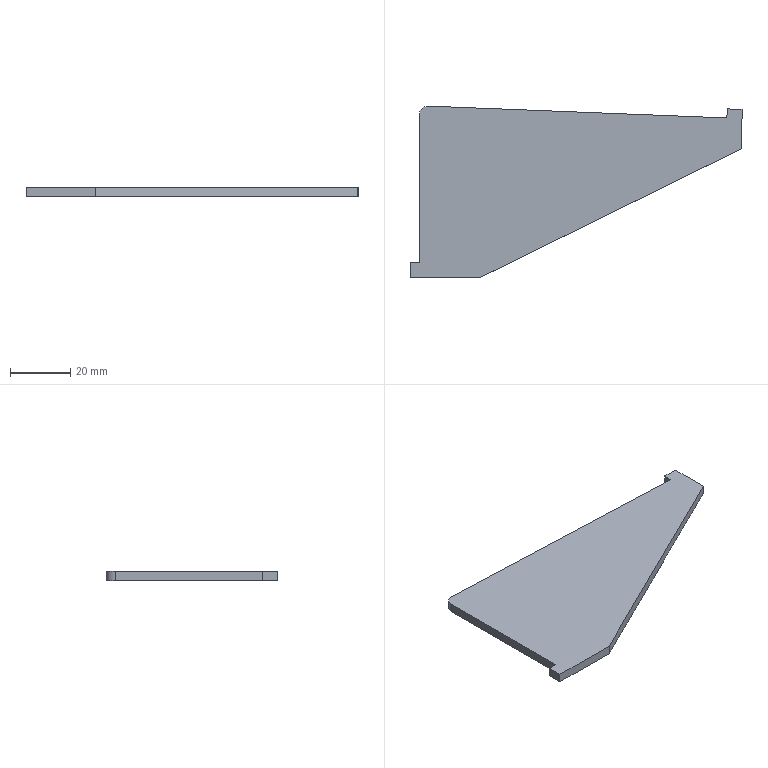Part | STEP file | TS-003-02 | 1 solid | 13 faces | box 109.897 x 56.866 x 3 mm | volume 12102 mm3 | plane 12 | cylinder 1 | commonest cylinder face diameters 6 x1
STEP:
#1=CARTESIAN_POINT('',(0.,0.,0.));
#2=DIRECTION('',(0.,0.,1.));
#3=DIRECTION('',(1.,0.,0.));
#4=AXIS2_PLACEMENT_3D('',#1,#2,#3);
#5=CARTESIAN_POINT('',(-4321.085,3720.403,0.));
#6=VERTEX_POINT('',#5);
#7=CARTESIAN_POINT('',(-4234.241,3763.152,0.));
#8=VERTEX_POINT('',#7);
#9=CARTESIAN_POINT('',(-4234.241,3763.152,0.));
#10=DIRECTION('',(0.8972,0.4416,0.));
#11=VECTOR('',#10,1.);
#12=LINE('',#9,#11);
#13=CARTESIAN_POINT('',(-4234.241,3763.152,-3.));
#14=DIRECTION('',(0.4416,-0.8972,0.));
#15=DIRECTION('',(0.8972,0.4416,0.));
#16=AXIS2_PLACEMENT_3D('',#13,#14,#15);
#17=PLANE('',#16);
#18=CARTESIAN_POINT('',(0.,3.));
#19=DIRECTION('',(1.,0.));
#20=VECTOR('',#19,1.);
#21=LINE('',#18,#20);
#22=(GEOMETRIC_REPRESENTATION_CONTEXT(2)PARAMETRIC_REPRESENTATION_CONTEXT()REPRESENTATION_CONTEXT('',''));
#23=DEFINITIONAL_REPRESENTATION('',(#21),#22);
#24=PCURVE('',#17,#23);
#25=CARTESIAN_POINT('',(-4338.085,3774.268,0.));
#26=DIRECTION('',(0.,0.,-1.));
#27=DIRECTION('',(-1.,0.,0.));
#28=AXIS2_PLACEMENT_3D('',#25,#26,#27);
#29=PLANE('',#28);
#30=CARTESIAN_POINT('',(-103.844,-11.117));
#31=DIRECTION('',(-0.8972,0.4416));
#32=VECTOR('',#31,1.);
#33=LINE('',#30,#32);
#34=(GEOMETRIC_REPRESENTATION_CONTEXT(2)PARAMETRIC_REPRESENTATION_CONTEXT()REPRESENTATION_CONTEXT('',''));
#35=DEFINITIONAL_REPRESENTATION('',(#33),#34);
#36=PCURVE('',#29,#35);
#37=SURFACE_CURVE('',#12,(#24,#36),.PCURVE_S1.);
#38=EDGE_CURVE('',#6,#8,#37,.T.);
#39=ORIENTED_EDGE('',*,*,#38,.F.);
#40=CARTESIAN_POINT('',(-4321.085,3720.403,-3.));
#41=VERTEX_POINT('',#40);
#42=CARTESIAN_POINT('',(-4321.085,3720.403,-3.));
#43=DIRECTION('',(0.,0.,1.));
#44=VECTOR('',#43,1.);
#45=LINE('',#42,#44);
#46=CARTESIAN_POINT('',(-96.795,0.));
#47=DIRECTION('',(0.,1.));
#48=VECTOR('',#47,1.);
#49=LINE('',#46,#48);
#50=(GEOMETRIC_REPRESENTATION_CONTEXT(2)PARAMETRIC_REPRESENTATION_CONTEXT()REPRESENTATION_CONTEXT('',''));
#51=DEFINITIONAL_REPRESENTATION('',(#49),#50);
#52=PCURVE('',#17,#51);
#53=CARTESIAN_POINT('',(-4321.085,3720.403,-3.));
#54=DIRECTION('',(0.,-1.,0.));
#55=DIRECTION('',(0.,0.,-1.));
#56=AXIS2_PLACEMENT_3D('',#53,#54,#55);
#57=PLANE('',#56);
#58=CARTESIAN_POINT('',(0.,0.));
#59=DIRECTION('',(-1.,0.));
#60=VECTOR('',#59,1.);
#61=LINE('',#58,#60);
#62=(GEOMETRIC_REPRESENTATION_CONTEXT(2)PARAMETRIC_REPRESENTATION_CONTEXT()REPRESENTATION_CONTEXT('',''));
#63=DEFINITIONAL_REPRESENTATION('',(#61),#62);
#64=PCURVE('',#57,#63);
#65=SURFACE_CURVE('',#45,(#52,#64),.PCURVE_S1.);
#66=EDGE_CURVE('',#41,#6,#65,.T.);
#67=ORIENTED_EDGE('',*,*,#66,.F.);
#68=CARTESIAN_POINT('',(-4234.241,3763.152,-3.));
#69=VERTEX_POINT('',#68);
#70=CARTESIAN_POINT('',(-4234.241,3763.152,-3.));
#71=DIRECTION('',(0.8972,0.4416,0.));
#72=VECTOR('',#71,1.);
#73=LINE('',#70,#72);
#74=CARTESIAN_POINT('',(0.,0.));
#75=DIRECTION('',(1.,0.));
#76=VECTOR('',#75,1.);
#77=LINE('',#74,#76);
#78=(GEOMETRIC_REPRESENTATION_CONTEXT(2)PARAMETRIC_REPRESENTATION_CONTEXT()REPRESENTATION_CONTEXT('',''));
#79=DEFINITIONAL_REPRESENTATION('',(#77),#78);
#80=PCURVE('',#17,#79);
#81=CARTESIAN_POINT('',(-4338.085,3774.268,-3.));
#82=DIRECTION('',(0.,0.,-1.));
#83=DIRECTION('',(-1.,0.,0.));
#84=AXIS2_PLACEMENT_3D('',#81,#82,#83);
#85=PLANE('',#84);
#86=CARTESIAN_POINT('',(-103.844,-11.117));
#87=DIRECTION('',(-0.8972,0.4416));
#88=VECTOR('',#87,1.);
#89=LINE('',#86,#88);
#90=(GEOMETRIC_REPRESENTATION_CONTEXT(2)PARAMETRIC_REPRESENTATION_CONTEXT()REPRESENTATION_CONTEXT('',''));
#91=DEFINITIONAL_REPRESENTATION('',(#89),#90);
#92=PCURVE('',#85,#91);
#93=SURFACE_CURVE('',#73,(#80,#92),.PCURVE_S1.);
#94=EDGE_CURVE('',#41,#69,#93,.T.);
#95=ORIENTED_EDGE('',*,*,#94,.T.);
#96=CARTESIAN_POINT('',(-4234.241,3763.152,-3.));
#97=DIRECTION('',(0.,0.,1.));
#98=VECTOR('',#97,1.);
#99=LINE('',#96,#98);
#100=CARTESIAN_POINT('',(0.,0.));
#101=DIRECTION('',(0.,1.));
#102=VECTOR('',#101,1.);
#103=LINE('',#100,#102);
#104=(GEOMETRIC_REPRESENTATION_CONTEXT(2)PARAMETRIC_REPRESENTATION_CONTEXT()REPRESENTATION_CONTEXT('',''));
#105=DEFINITIONAL_REPRESENTATION('',(#103),#104);
#106=PCURVE('',#17,#105);
#107=CARTESIAN_POINT('',(-4234.188,3773.152,-3.));
#108=DIRECTION('',(1.,-0.005262,0.));
#109=DIRECTION('',(0.005262,1.,0.));
#110=AXIS2_PLACEMENT_3D('',#107,#108,#109);
#111=PLANE('',#110);
#112=CARTESIAN_POINT('',(-10.,0.));
#113=DIRECTION('',(0.,1.));
#114=VECTOR('',#113,1.);
#115=LINE('',#112,#114);
#116=(GEOMETRIC_REPRESENTATION_CONTEXT(2)PARAMETRIC_REPRESENTATION_CONTEXT()REPRESENTATION_CONTEXT('',''));
#117=DEFINITIONAL_REPRESENTATION('',(#115),#116);
#118=PCURVE('',#111,#117);
#119=SURFACE_CURVE('',#99,(#106,#118),.PCURVE_S1.);
#120=EDGE_CURVE('',#69,#8,#119,.T.);
#121=ORIENTED_EDGE('',*,*,#120,.T.);
#122=EDGE_LOOP('',(#39,#67,#95,#121));
#123=FACE_BOUND('',#122,.T.);
#124=ADVANCED_FACE('',(#123),#17,.T.);
#125=CARTESIAN_POINT('',(-4344.085,3720.403,0.));
#126=VERTEX_POINT('',#125);
#127=CARTESIAN_POINT('',(-4321.085,3720.403,0.));
#128=DIRECTION('',(1.,0.,0.));
#129=VECTOR('',#128,1.);
#130=LINE('',#127,#129);
#131=CARTESIAN_POINT('',(-3.,0.));
#132=DIRECTION('',(0.,1.));
#133=VECTOR('',#132,1.);
#134=LINE('',#131,#133);
#135=(GEOMETRIC_REPRESENTATION_CONTEXT(2)PARAMETRIC_REPRESENTATION_CONTEXT()REPRESENTATION_CONTEXT('',''));
#136=DEFINITIONAL_REPRESENTATION('',(#134),#135);
#137=PCURVE('',#57,#136);
#138=CARTESIAN_POINT('',(-17.,-53.866));
#139=DIRECTION('',(-1.,0.));
#140=VECTOR('',#139,1.);
#141=LINE('',#138,#140);
#142=(GEOMETRIC_REPRESENTATION_CONTEXT(2)PARAMETRIC_REPRESENTATION_CONTEXT()REPRESENTATION_CONTEXT('',''));
#143=DEFINITIONAL_REPRESENTATION('',(#141),#142);
#144=PCURVE('',#29,#143);
#145=SURFACE_CURVE('',#130,(#137,#144),.PCURVE_S1.);
#146=EDGE_CURVE('',#126,#6,#145,.T.);
#147=ORIENTED_EDGE('',*,*,#146,.F.);
#148=CARTESIAN_POINT('',(-4344.085,3720.403,-3.));
#149=VERTEX_POINT('',#148);
#150=CARTESIAN_POINT('',(-4344.085,3720.403,-3.));
#151=DIRECTION('',(0.,0.,1.));
#152=VECTOR('',#151,1.);
#153=LINE('',#150,#152);
#154=CARTESIAN_POINT('',(0.,-23.));
#155=DIRECTION('',(-1.,0.));
#156=VECTOR('',#155,1.);
#157=LINE('',#154,#156);
#158=(GEOMETRIC_REPRESENTATION_CONTEXT(2)PARAMETRIC_REPRESENTATION_CONTEXT()REPRESENTATION_CONTEXT('',''));
#159=DEFINITIONAL_REPRESENTATION('',(#157),#158);
#160=PCURVE('',#57,#159);
#161=CARTESIAN_POINT('',(-4344.085,3720.403,-3.));
#162=DIRECTION('',(-1.,0.,0.));
#163=DIRECTION('',(0.,0.,1.));
#164=AXIS2_PLACEMENT_3D('',#161,#162,#163);
#165=PLANE('',#164);
#166=CARTESIAN_POINT('',(0.,0.));
#167=DIRECTION('',(1.,0.));
#168=VECTOR('',#167,1.);
#169=LINE('',#166,#168);
#170=(GEOMETRIC_REPRESENTATION_CONTEXT(2)PARAMETRIC_REPRESENTATION_CONTEXT()REPRESENTATION_CONTEXT('',''));
#171=DEFINITIONAL_REPRESENTATION('',(#169),#170);
#172=PCURVE('',#165,#171);
#173=SURFACE_CURVE('',#153,(#160,#172),.PCURVE_S1.);
#174=EDGE_CURVE('',#149,#126,#173,.T.);
#175=ORIENTED_EDGE('',*,*,#174,.F.);
#176=CARTESIAN_POINT('',(-4321.085,3720.403,-3.));
#177=DIRECTION('',(1.,0.,0.));
#178=VECTOR('',#177,1.);
#179=LINE('',#176,#178);
#180=CARTESIAN_POINT('',(0.,0.));
#181=DIRECTION('',(0.,1.));
#182=VECTOR('',#181,1.);
#183=LINE('',#180,#182);
#184=(GEOMETRIC_REPRESENTATION_CONTEXT(2)PARAMETRIC_REPRESENTATION_CONTEXT()REPRESENTATION_CONTEXT('',''));
#185=DEFINITIONAL_REPRESENTATION('',(#183),#184);
#186=PCURVE('',#57,#185);
#187=CARTESIAN_POINT('',(-17.,-53.866));
#188=DIRECTION('',(-1.,0.));
#189=VECTOR('',#188,1.);
#190=LINE('',#187,#189);
#191=(GEOMETRIC_REPRESENTATION_CONTEXT(2)PARAMETRIC_REPRESENTATION_CONTEXT()REPRESENTATION_CONTEXT('',''));
#192=DEFINITIONAL_REPRESENTATION('',(#190),#191);
#193=PCURVE('',#85,#192);
#194=SURFACE_CURVE('',#179,(#186,#193),.PCURVE_S1.);
#195=EDGE_CURVE('',#149,#41,#194,.T.);
#196=ORIENTED_EDGE('',*,*,#195,.T.);
#197=ORIENTED_EDGE('',*,*,#66,.T.);
#198=EDGE_LOOP('',(#147,#175,#196,#197));
#199=FACE_BOUND('',#198,.T.);
#200=ADVANCED_FACE('',(#199),#57,.T.);
#201=CARTESIAN_POINT('',(-4341.085,3725.403,-3.));
#202=VERTEX_POINT('',#201);
#203=CARTESIAN_POINT('',(-4341.085,3725.403,0.));
#204=VERTEX_POINT('',#203);
#205=CARTESIAN_POINT('',(-4341.085,3725.403,-3.));
#206=DIRECTION('',(0.,0.,1.));
#207=VECTOR('',#206,1.);
#208=LINE('',#205,#207);
#209=CARTESIAN_POINT('',(-4341.085,3720.403,-3.));
#210=DIRECTION('',(-1.,0.,0.));
#211=DIRECTION('',(0.,0.,1.));
#212=AXIS2_PLACEMENT_3D('',#209,#210,#211);
#213=PLANE('',#212);
#214=CARTESIAN_POINT('',(0.,5.));
#215=DIRECTION('',(1.,0.));
#216=VECTOR('',#215,1.);
#217=LINE('',#214,#216);
#218=(GEOMETRIC_REPRESENTATION_CONTEXT(2)PARAMETRIC_REPRESENTATION_CONTEXT()REPRESENTATION_CONTEXT('',''));
#219=DEFINITIONAL_REPRESENTATION('',(#217),#218);
#220=PCURVE('',#213,#219);
#221=CARTESIAN_POINT('',(-4341.085,3725.403,-3.));
#222=DIRECTION('',(0.,1.,0.));
#223=DIRECTION('',(0.,0.,1.));
#224=AXIS2_PLACEMENT_3D('',#221,#222,#223);
#225=PLANE('',#224);
#226=CARTESIAN_POINT('',(0.,0.));
#227=DIRECTION('',(1.,0.));
#228=VECTOR('',#227,1.);
#229=LINE('',#226,#228);
#230=(GEOMETRIC_REPRESENTATION_CONTEXT(2)PARAMETRIC_REPRESENTATION_CONTEXT()REPRESENTATION_CONTEXT('',''));
#231=DEFINITIONAL_REPRESENTATION('',(#229),#230);
#232=PCURVE('',#225,#231);
#233=SURFACE_CURVE('',#208,(#220,#232),.PCURVE_S1.);
#234=EDGE_CURVE('',#202,#204,#233,.T.);
#235=ORIENTED_EDGE('',*,*,#234,.T.);
#236=CARTESIAN_POINT('',(-4341.085,3774.268,0.));
#237=VERTEX_POINT('',#236);
#238=CARTESIAN_POINT('',(-4341.085,3720.403,0.));
#239=DIRECTION('',(0.,-1.,0.));
#240=VECTOR('',#239,1.);
#241=LINE('',#238,#240);
#242=CARTESIAN_POINT('',(3.,0.));
#243=DIRECTION('',(0.,-1.));
#244=VECTOR('',#243,1.);
#245=LINE('',#242,#244);
#246=(GEOMETRIC_REPRESENTATION_CONTEXT(2)PARAMETRIC_REPRESENTATION_CONTEXT()REPRESENTATION_CONTEXT('',''));
#247=DEFINITIONAL_REPRESENTATION('',(#245),#246);
#248=PCURVE('',#213,#247);
#249=CARTESIAN_POINT('',(3.,-53.866));
#250=DIRECTION('',(0.,-1.));
#251=VECTOR('',#250,1.);
#252=LINE('',#249,#251);
#253=(GEOMETRIC_REPRESENTATION_CONTEXT(2)PARAMETRIC_REPRESENTATION_CONTEXT()REPRESENTATION_CONTEXT('',''));
#254=DEFINITIONAL_REPRESENTATION('',(#252),#253);
#255=PCURVE('',#29,#254);
#256=SURFACE_CURVE('',#241,(#248,#255),.PCURVE_S1.);
#257=EDGE_CURVE('',#237,#204,#256,.T.);
#258=ORIENTED_EDGE('',*,*,#257,.F.);
#259=CARTESIAN_POINT('',(-4341.085,3774.268,-3.));
#260=VERTEX_POINT('',#259);
#261=CARTESIAN_POINT('',(-4341.085,3774.268,-3.));
#262=DIRECTION('',(0.,0.,1.));
#263=VECTOR('',#262,1.);
#264=LINE('',#261,#263);
#265=CARTESIAN_POINT('',(0.,53.866));
#266=DIRECTION('',(1.,0.));
#267=VECTOR('',#266,1.);
#268=LINE('',#265,#267);
#269=(GEOMETRIC_REPRESENTATION_CONTEXT(2)PARAMETRIC_REPRESENTATION_CONTEXT()REPRESENTATION_CONTEXT('',''));
#270=DEFINITIONAL_REPRESENTATION('',(#268),#269);
#271=PCURVE('',#213,#270);
#272=CARTESIAN_POINT('',(-4338.085,3774.268,-3.));
#273=DIRECTION('',(0.,0.,1.));
#274=DIRECTION('',(1.,0.,0.));
#275=AXIS2_PLACEMENT_3D('',#272,#273,#274);
#276=CYLINDRICAL_SURFACE('',#275,3.);
#277=CARTESIAN_POINT('',(3.142,0.));
#278=DIRECTION('',(0.,1.));
#279=VECTOR('',#278,1.);
#280=LINE('',#277,#279);
#281=(GEOMETRIC_REPRESENTATION_CONTEXT(2)PARAMETRIC_REPRESENTATION_CONTEXT()REPRESENTATION_CONTEXT('',''));
#282=DEFINITIONAL_REPRESENTATION('',(#280),#281);
#283=PCURVE('',#276,#282);
#284=SURFACE_CURVE('',#264,(#271,#283),.PCURVE_S1.);
#285=EDGE_CURVE('',#260,#237,#284,.T.);
#286=ORIENTED_EDGE('',*,*,#285,.F.);
#287=CARTESIAN_POINT('',(-4341.085,3720.403,-3.));
#288=DIRECTION('',(0.,-1.,0.));
#289=VECTOR('',#288,1.);
#290=LINE('',#287,#289);
#291=CARTESIAN_POINT('',(0.,0.));
#292=DIRECTION('',(0.,-1.));
#293=VECTOR('',#292,1.);
#294=LINE('',#291,#293);
#295=(GEOMETRIC_REPRESENTATION_CONTEXT(2)PARAMETRIC_REPRESENTATION_CONTEXT()REPRESENTATION_CONTEXT('',''));
#296=DEFINITIONAL_REPRESENTATION('',(#294),#295);
#297=PCURVE('',#213,#296);
#298=CARTESIAN_POINT('',(3.,-53.866));
#299=DIRECTION('',(0.,-1.));
#300=VECTOR('',#299,1.);
#301=LINE('',#298,#300);
#302=(GEOMETRIC_REPRESENTATION_CONTEXT(2)PARAMETRIC_REPRESENTATION_CONTEXT()REPRESENTATION_CONTEXT('',''));
#303=DEFINITIONAL_REPRESENTATION('',(#301),#302);
#304=PCURVE('',#85,#303);
#305=SURFACE_CURVE('',#290,(#297,#304),.PCURVE_S1.);
#306=EDGE_CURVE('',#260,#202,#305,.T.);
#307=ORIENTED_EDGE('',*,*,#306,.T.);
#308=EDGE_LOOP('',(#235,#258,#286,#307));
#309=FACE_BOUND('',#308,.T.);
#310=ADVANCED_FACE('',(#309),#213,.T.);
#311=CARTESIAN_POINT('',(-4338.019,3777.268,0.));
#312=VERTEX_POINT('',#311);
#313=CARTESIAN_POINT('',(-4338.085,3774.268,0.));
#314=DIRECTION('',(0.,0.,1.));
#315=DIRECTION('',(-1.,0.,0.));
#316=AXIS2_PLACEMENT_3D('',#313,#314,#315);
#317=CIRCLE('',#316,3.);
#318=CARTESIAN_POINT('',(-3.142,3.));
#319=DIRECTION('',(1.,0.));
#320=VECTOR('',#319,1.);
#321=LINE('',#318,#320);
#322=(GEOMETRIC_REPRESENTATION_CONTEXT(2)PARAMETRIC_REPRESENTATION_CONTEXT()REPRESENTATION_CONTEXT('',''));
#323=DEFINITIONAL_REPRESENTATION('',(#321),#322);
#324=PCURVE('',#276,#323);
#325=CARTESIAN_POINT('',(3.,0.));
#326=CARTESIAN_POINT('',(3.,-5.196));
#327=CARTESIAN_POINT('',(-1.5,-2.598));
#328=CARTESIAN_POINT('',(-6.,0.));
#329=CARTESIAN_POINT('',(-1.5,2.598));
#330=CARTESIAN_POINT('',(3.,5.196));
#331=CARTESIAN_POINT('',(3.,0.));
#332=(BOUNDED_CURVE()B_SPLINE_CURVE(2,(#325,#326,#327,#328,#329,#330,#331),.UNSPECIFIED.,.T.,.F.)B_SPLINE_CURVE_WITH_KNOTS((1,2,2,2,2,1),(-2.094,0.,2.094,4.189,6.283,8.378),.UNSPECIFIED.)CURVE()GEOMETRIC_REPRESENTATION_ITEM()RATIONAL_B_SPLINE_CURVE((1.,0.5,1.,0.5,1.,0.5,1.))REPRESENTATION_ITEM(''));
#333=(GEOMETRIC_REPRESENTATION_CONTEXT(2)PARAMETRIC_REPRESENTATION_CONTEXT()REPRESENTATION_CONTEXT('',''));
#334=DEFINITIONAL_REPRESENTATION('',(#332),#333);
#335=PCURVE('',#29,#334);
#336=SURFACE_CURVE('',#317,(#324,#335),.PCURVE_S1.);
#337=EDGE_CURVE('',#312,#237,#336,.T.);
#338=ORIENTED_EDGE('',*,*,#337,.F.);
#339=CARTESIAN_POINT('',(-4338.019,3777.268,-3.));
#340=VERTEX_POINT('',#339);
#341=CARTESIAN_POINT('',(-4338.019,3777.268,-3.));
#342=DIRECTION('',(0.,0.,1.));
#343=VECTOR('',#342,1.);
#344=LINE('',#341,#343);
#345=CARTESIAN_POINT('',(1.549,0.));
#346=DIRECTION('',(0.,1.));
#347=VECTOR('',#346,1.);
#348=LINE('',#345,#347);
#349=(GEOMETRIC_REPRESENTATION_CONTEXT(2)PARAMETRIC_REPRESENTATION_CONTEXT()REPRESENTATION_CONTEXT('',''));
#350=DEFINITIONAL_REPRESENTATION('',(#348),#349);
#351=PCURVE('',#276,#350);
#352=CARTESIAN_POINT('',(-4338.019,3777.268,-3.));
#353=DIRECTION('',(0.03961,0.9992,0.));
#354=DIRECTION('',(-0.9992,0.03961,0.));
#355=AXIS2_PLACEMENT_3D('',#352,#353,#354);
#356=PLANE('',#355);
#357=CARTESIAN_POINT('',(0.,0.));
#358=DIRECTION('',(0.,1.));
#359=VECTOR('',#358,1.);
#360=LINE('',#357,#359);
#361=(GEOMETRIC_REPRESENTATION_CONTEXT(2)PARAMETRIC_REPRESENTATION_CONTEXT()REPRESENTATION_CONTEXT('',''));
#362=DEFINITIONAL_REPRESENTATION('',(#360),#361);
#363=PCURVE('',#356,#362);
#364=SURFACE_CURVE('',#344,(#351,#363),.PCURVE_S1.);
#365=EDGE_CURVE('',#340,#312,#364,.T.);
#366=ORIENTED_EDGE('',*,*,#365,.F.);
#367=CARTESIAN_POINT('',(-4338.085,3774.268,-3.));
#368=DIRECTION('',(0.,0.,1.));
#369=DIRECTION('',(-1.,0.,0.));
#370=AXIS2_PLACEMENT_3D('',#367,#368,#369);
#371=CIRCLE('',#370,3.);
#372=CARTESIAN_POINT('',(-3.142,0.));
#373=DIRECTION('',(1.,0.));
#374=VECTOR('',#373,1.);
#375=LINE('',#372,#374);
#376=(GEOMETRIC_REPRESENTATION_CONTEXT(2)PARAMETRIC_REPRESENTATION_CONTEXT()REPRESENTATION_CONTEXT('',''));
#377=DEFINITIONAL_REPRESENTATION('',(#375),#376);
#378=PCURVE('',#276,#377);
#379=CARTESIAN_POINT('',(3.,0.));
#380=CARTESIAN_POINT('',(3.,-5.196));
#381=CARTESIAN_POINT('',(-1.5,-2.598));
#382=CARTESIAN_POINT('',(-6.,0.));
#383=CARTESIAN_POINT('',(-1.5,2.598));
#384=CARTESIAN_POINT('',(3.,5.196));
#385=CARTESIAN_POINT('',(3.,0.));
#386=(BOUNDED_CURVE()B_SPLINE_CURVE(2,(#379,#380,#381,#382,#383,#384,#385),.UNSPECIFIED.,.T.,.F.)B_SPLINE_CURVE_WITH_KNOTS((1,2,2,2,2,1),(-2.094,0.,2.094,4.189,6.283,8.378),.UNSPECIFIED.)CURVE()GEOMETRIC_REPRESENTATION_ITEM()RATIONAL_B_SPLINE_CURVE((1.,0.5,1.,0.5,1.,0.5,1.))REPRESENTATION_ITEM(''));
#387=(GEOMETRIC_REPRESENTATION_CONTEXT(2)PARAMETRIC_REPRESENTATION_CONTEXT()REPRESENTATION_CONTEXT('',''));
#388=DEFINITIONAL_REPRESENTATION('',(#386),#387);
#389=PCURVE('',#85,#388);
#390=SURFACE_CURVE('',#371,(#378,#389),.PCURVE_S1.);
#391=EDGE_CURVE('',#340,#260,#390,.T.);
#392=ORIENTED_EDGE('',*,*,#391,.T.);
#393=ORIENTED_EDGE('',*,*,#285,.T.);
#394=EDGE_LOOP('',(#338,#366,#392,#393));
#395=FACE_BOUND('',#394,.T.);
#396=ADVANCED_FACE('',(#395),#276,.T.);
#397=CARTESIAN_POINT('',(-4239.188,3773.35,-3.));
#398=VERTEX_POINT('',#397);
#399=CARTESIAN_POINT('',(-4239.188,3773.35,0.));
#400=VERTEX_POINT('',#399);
#401=CARTESIAN_POINT('',(-4239.188,3773.35,-3.));
#402=DIRECTION('',(0.,0.,1.));
#403=VECTOR('',#402,1.);
#404=LINE('',#401,#403);
#405=CARTESIAN_POINT('',(-98.908,0.));
#406=DIRECTION('',(0.,1.));
#407=VECTOR('',#406,1.);
#408=LINE('',#405,#407);
#409=(GEOMETRIC_REPRESENTATION_CONTEXT(2)PARAMETRIC_REPRESENTATION_CONTEXT()REPRESENTATION_CONTEXT('',''));
#410=DEFINITIONAL_REPRESENTATION('',(#408),#409);
#411=PCURVE('',#356,#410);
#412=CARTESIAN_POINT('',(-4239.07,3776.348,-3.));
#413=DIRECTION('',(-0.9992,0.03961,0.));
#414=DIRECTION('',(-0.03961,-0.9992,0.));
#415=AXIS2_PLACEMENT_3D('',#412,#413,#414);
#416=PLANE('',#415);
#417=CARTESIAN_POINT('',(3.,0.));
#418=DIRECTION('',(0.,1.));
#419=VECTOR('',#418,1.);
#420=LINE('',#417,#419);
#421=(GEOMETRIC_REPRESENTATION_CONTEXT(2)PARAMETRIC_REPRESENTATION_CONTEXT()REPRESENTATION_CONTEXT('',''));
#422=DEFINITIONAL_REPRESENTATION('',(#420),#421);
#423=PCURVE('',#416,#422);
#424=SURFACE_CURVE('',#404,(#411,#423),.PCURVE_S1.);
#425=EDGE_CURVE('',#398,#400,#424,.T.);
#426=ORIENTED_EDGE('',*,*,#425,.F.);
#427=CARTESIAN_POINT('',(-4338.019,3777.268,-3.));
#428=DIRECTION('',(-0.9992,0.03961,0.));
#429=VECTOR('',#428,1.);
#430=LINE('',#427,#429);
#431=CARTESIAN_POINT('',(0.,0.));
#432=DIRECTION('',(1.,0.));
#433=VECTOR('',#432,1.);
#434=LINE('',#431,#433);
#435=(GEOMETRIC_REPRESENTATION_CONTEXT(2)PARAMETRIC_REPRESENTATION_CONTEXT()REPRESENTATION_CONTEXT('',''));
#436=DEFINITIONAL_REPRESENTATION('',(#434),#435);
#437=PCURVE('',#356,#436);
#438=CARTESIAN_POINT('',(-0.06649,2.999));
#439=DIRECTION('',(0.9992,0.03961));
#440=VECTOR('',#439,1.);
#441=LINE('',#438,#440);
#442=(GEOMETRIC_REPRESENTATION_CONTEXT(2)PARAMETRIC_REPRESENTATION_CONTEXT()REPRESENTATION_CONTEXT('',''));
#443=DEFINITIONAL_REPRESENTATION('',(#441),#442);
#444=PCURVE('',#85,#443);
#445=SURFACE_CURVE('',#430,(#437,#444),.PCURVE_S1.);
#446=EDGE_CURVE('',#398,#340,#445,.T.);
#447=ORIENTED_EDGE('',*,*,#446,.T.);
#448=ORIENTED_EDGE('',*,*,#365,.T.);
#449=CARTESIAN_POINT('',(-4338.019,3777.268,0.));
#450=DIRECTION('',(-0.9992,0.03961,0.));
#451=VECTOR('',#450,1.);
#452=LINE('',#449,#451);
#453=CARTESIAN_POINT('',(0.,3.));
#454=DIRECTION('',(1.,0.));
#455=VECTOR('',#454,1.);
#456=LINE('',#453,#455);
#457=(GEOMETRIC_REPRESENTATION_CONTEXT(2)PARAMETRIC_REPRESENTATION_CONTEXT()REPRESENTATION_CONTEXT('',''));
#458=DEFINITIONAL_REPRESENTATION('',(#456),#457);
#459=PCURVE('',#356,#458);
#460=CARTESIAN_POINT('',(-0.06649,2.999));
#461=DIRECTION('',(0.9992,0.03961));
#462=VECTOR('',#461,1.);
#463=LINE('',#460,#462);
#464=(GEOMETRIC_REPRESENTATION_CONTEXT(2)PARAMETRIC_REPRESENTATION_CONTEXT()REPRESENTATION_CONTEXT('',''));
#465=DEFINITIONAL_REPRESENTATION('',(#463),#464);
#466=PCURVE('',#29,#465);
#467=SURFACE_CURVE('',#452,(#459,#466),.PCURVE_S1.);
#468=EDGE_CURVE('',#400,#312,#467,.T.);
#469=ORIENTED_EDGE('',*,*,#468,.F.);
#470=EDGE_LOOP('',(#426,#447,#448,#469));
#471=FACE_BOUND('',#470,.T.);
#472=ADVANCED_FACE('',(#471),#356,.T.);
#473=CARTESIAN_POINT('',(-4234.188,3773.152,0.));
#474=VERTEX_POINT('',#473);
#475=CARTESIAN_POINT('',(-4234.188,3773.152,0.));
#476=DIRECTION('',(0.005262,1.,0.));
#477=VECTOR('',#476,1.);
#478=LINE('',#475,#477);
#479=CARTESIAN_POINT('',(0.,3.));
#480=DIRECTION('',(1.,0.));
#481=VECTOR('',#480,1.);
#482=LINE('',#479,#481);
#483=(GEOMETRIC_REPRESENTATION_CONTEXT(2)PARAMETRIC_REPRESENTATION_CONTEXT()REPRESENTATION_CONTEXT('',''));
#484=DEFINITIONAL_REPRESENTATION('',(#482),#483);
#485=PCURVE('',#111,#484);
#486=CARTESIAN_POINT('',(-103.897,-1.117));
#487=DIRECTION('',(-0.005262,1.));
#488=VECTOR('',#487,1.);
#489=LINE('',#486,#488);
#490=(GEOMETRIC_REPRESENTATION_CONTEXT(2)PARAMETRIC_REPRESENTATION_CONTEXT()REPRESENTATION_CONTEXT('',''));
#491=DEFINITIONAL_REPRESENTATION('',(#489),#490);
#492=PCURVE('',#29,#491);
#493=SURFACE_CURVE('',#478,(#485,#492),.PCURVE_S1.);
#494=EDGE_CURVE('',#8,#474,#493,.T.);
#495=ORIENTED_EDGE('',*,*,#494,.F.);
#496=ORIENTED_EDGE('',*,*,#120,.F.);
#497=CARTESIAN_POINT('',(-4234.188,3773.152,-3.));
#498=VERTEX_POINT('',#497);
#499=CARTESIAN_POINT('',(-4234.188,3773.152,-3.));
#500=DIRECTION('',(0.005262,1.,0.));
#501=VECTOR('',#500,1.);
#502=LINE('',#499,#501);
#503=CARTESIAN_POINT('',(0.,0.));
#504=DIRECTION('',(1.,0.));
#505=VECTOR('',#504,1.);
#506=LINE('',#503,#505);
#507=(GEOMETRIC_REPRESENTATION_CONTEXT(2)PARAMETRIC_REPRESENTATION_CONTEXT()REPRESENTATION_CONTEXT('',''));
#508=DEFINITIONAL_REPRESENTATION('',(#506),#507);
#509=PCURVE('',#111,#508);
#510=CARTESIAN_POINT('',(-103.897,-1.117));
#511=DIRECTION('',(-0.005262,1.));
#512=VECTOR('',#511,1.);
#513=LINE('',#510,#512);
#514=(GEOMETRIC_REPRESENTATION_CONTEXT(2)PARAMETRIC_REPRESENTATION_CONTEXT()REPRESENTATION_CONTEXT('',''));
#515=DEFINITIONAL_REPRESENTATION('',(#513),#514);
#516=PCURVE('',#85,#515);
#517=SURFACE_CURVE('',#502,(#509,#516),.PCURVE_S1.);
#518=EDGE_CURVE('',#69,#498,#517,.T.);
#519=ORIENTED_EDGE('',*,*,#518,.T.);
#520=CARTESIAN_POINT('',(-4234.188,3773.152,-3.));
#521=DIRECTION('',(0.,0.,1.));
#522=VECTOR('',#521,1.);
#523=LINE('',#520,#522);
#524=CARTESIAN_POINT('',(0.,0.));
#525=DIRECTION('',(0.,1.));
#526=VECTOR('',#525,1.);
#527=LINE('',#524,#526);
#528=(GEOMETRIC_REPRESENTATION_CONTEXT(2)PARAMETRIC_REPRESENTATION_CONTEXT()REPRESENTATION_CONTEXT('',''));
#529=DEFINITIONAL_REPRESENTATION('',(#527),#528);
#530=PCURVE('',#111,#529);
#531=CARTESIAN_POINT('',(-4234.188,3773.152,-3.));
#532=DIRECTION('',(1.,0.,0.));
#533=DIRECTION('',(0.,0.,-1.));
#534=AXIS2_PLACEMENT_3D('',#531,#532,#533);
#535=PLANE('',#534);
#536=CARTESIAN_POINT('',(0.,0.));
#537=DIRECTION('',(-1.,0.));
#538=VECTOR('',#537,1.);
#539=LINE('',#536,#538);
#540=(GEOMETRIC_REPRESENTATION_CONTEXT(2)PARAMETRIC_REPRESENTATION_CONTEXT()REPRESENTATION_CONTEXT('',''));
#541=DEFINITIONAL_REPRESENTATION('',(#539),#540);
#542=PCURVE('',#535,#541);
#543=SURFACE_CURVE('',#523,(#530,#542),.PCURVE_S1.);
#544=EDGE_CURVE('',#498,#474,#543,.T.);
#545=ORIENTED_EDGE('',*,*,#544,.T.);
#546=EDGE_LOOP('',(#495,#496,#519,#545));
#547=FACE_BOUND('',#546,.T.);
#548=ADVANCED_FACE('',(#547),#111,.T.);
#549=ORIENTED_EDGE('',*,*,#94,.F.);
#550=ORIENTED_EDGE('',*,*,#195,.F.);
#551=CARTESIAN_POINT('',(-4344.085,3725.403,-3.));
#552=VERTEX_POINT('',#551);
#553=CARTESIAN_POINT('',(-4344.085,3720.403,-3.));
#554=DIRECTION('',(0.,-1.,0.));
#555=VECTOR('',#554,1.);
#556=LINE('',#553,#555);
#557=CARTESIAN_POINT('',(6.,-53.866));
#558=DIRECTION('',(0.,-1.));
#559=VECTOR('',#558,1.);
#560=LINE('',#557,#559);
#561=(GEOMETRIC_REPRESENTATION_CONTEXT(2)PARAMETRIC_REPRESENTATION_CONTEXT()REPRESENTATION_CONTEXT('',''));
#562=DEFINITIONAL_REPRESENTATION('',(#560),#561);
#563=PCURVE('',#85,#562);
#564=CARTESIAN_POINT('',(0.,0.));
#565=DIRECTION('',(0.,-1.));
#566=VECTOR('',#565,1.);
#567=LINE('',#564,#566);
#568=(GEOMETRIC_REPRESENTATION_CONTEXT(2)PARAMETRIC_REPRESENTATION_CONTEXT()REPRESENTATION_CONTEXT('',''));
#569=DEFINITIONAL_REPRESENTATION('',(#567),#568);
#570=PCURVE('',#165,#569);
#571=SURFACE_CURVE('',#556,(#563,#570),.PCURVE_S1.);
#572=EDGE_CURVE('',#552,#149,#571,.T.);
#573=ORIENTED_EDGE('',*,*,#572,.F.);
#574=CARTESIAN_POINT('',(-4341.085,3725.403,-3.));
#575=DIRECTION('',(-1.,0.,0.));
#576=VECTOR('',#575,1.);
#577=LINE('',#574,#576);
#578=CARTESIAN_POINT('',(3.,-48.866));
#579=DIRECTION('',(1.,0.));
#580=VECTOR('',#579,1.);
#581=LINE('',#578,#580);
#582=(GEOMETRIC_REPRESENTATION_CONTEXT(2)PARAMETRIC_REPRESENTATION_CONTEXT()REPRESENTATION_CONTEXT('',''));
#583=DEFINITIONAL_REPRESENTATION('',(#581),#582);
#584=PCURVE('',#85,#583);
#585=CARTESIAN_POINT('',(0.,0.));
#586=DIRECTION('',(0.,-1.));
#587=VECTOR('',#586,1.);
#588=LINE('',#585,#587);
#589=(GEOMETRIC_REPRESENTATION_CONTEXT(2)PARAMETRIC_REPRESENTATION_CONTEXT()REPRESENTATION_CONTEXT('',''));
#590=DEFINITIONAL_REPRESENTATION('',(#588),#589);
#591=PCURVE('',#225,#590);
#592=SURFACE_CURVE('',#577,(#584,#591),.PCURVE_S1.);
#593=EDGE_CURVE('',#202,#552,#592,.T.);
#594=ORIENTED_EDGE('',*,*,#593,.F.);
#595=ORIENTED_EDGE('',*,*,#306,.F.);
#596=ORIENTED_EDGE('',*,*,#391,.F.);
#597=ORIENTED_EDGE('',*,*,#446,.F.);
#598=CARTESIAN_POINT('',(-4239.07,3776.348,-3.));
#599=VERTEX_POINT('',#598);
#600=CARTESIAN_POINT('',(-4239.07,3776.348,-3.));
#601=DIRECTION('',(-0.03961,-0.9992,0.));
#602=VECTOR('',#601,1.);
#603=LINE('',#600,#602);
#604=CARTESIAN_POINT('',(-99.015,2.079));
#605=DIRECTION('',(0.03961,-0.9992));
#606=VECTOR('',#605,1.);
#607=LINE('',#604,#606);
#608=(GEOMETRIC_REPRESENTATION_CONTEXT(2)PARAMETRIC_REPRESENTATION_CONTEXT()REPRESENTATION_CONTEXT('',''));
#609=DEFINITIONAL_REPRESENTATION('',(#607),#608);
#610=PCURVE('',#85,#609);
#611=CARTESIAN_POINT('',(0.,0.));
#612=DIRECTION('',(1.,0.));
#613=VECTOR('',#612,1.);
#614=LINE('',#611,#613);
#615=(GEOMETRIC_REPRESENTATION_CONTEXT(2)PARAMETRIC_REPRESENTATION_CONTEXT()REPRESENTATION_CONTEXT('',''));
#616=DEFINITIONAL_REPRESENTATION('',(#614),#615);
#617=PCURVE('',#416,#616);
#618=SURFACE_CURVE('',#603,(#610,#617),.PCURVE_S1.);
#619=EDGE_CURVE('',#599,#398,#618,.T.);
#620=ORIENTED_EDGE('',*,*,#619,.F.);
#621=CARTESIAN_POINT('',(-4234.188,3776.154,-3.));
#622=VERTEX_POINT('',#621);
#623=CARTESIAN_POINT('',(-4234.188,3776.154,-3.));
#624=DIRECTION('',(-0.9992,0.03961,0.));
#625=VECTOR('',#624,1.);
#626=LINE('',#623,#625);
#627=CARTESIAN_POINT('',(-103.897,1.886));
#628=DIRECTION('',(0.9992,0.03961));
#629=VECTOR('',#628,1.);
#630=LINE('',#627,#629);
#631=(GEOMETRIC_REPRESENTATION_CONTEXT(2)PARAMETRIC_REPRESENTATION_CONTEXT()REPRESENTATION_CONTEXT('',''));
#632=DEFINITIONAL_REPRESENTATION('',(#630),#631);
#633=PCURVE('',#85,#632);
#634=CARTESIAN_POINT('',(-4234.188,3776.154,-3.));
#635=DIRECTION('',(0.03961,0.9992,0.));
#636=DIRECTION('',(-0.9992,0.03961,0.));
#637=AXIS2_PLACEMENT_3D('',#634,#635,#636);
#638=PLANE('',#637);
#639=CARTESIAN_POINT('',(0.,0.));
#640=DIRECTION('',(1.,0.));
#641=VECTOR('',#640,1.);
#642=LINE('',#639,#641);
#643=(GEOMETRIC_REPRESENTATION_CONTEXT(2)PARAMETRIC_REPRESENTATION_CONTEXT()REPRESENTATION_CONTEXT('',''));
#644=DEFINITIONAL_REPRESENTATION('',(#642),#643);
#645=PCURVE('',#638,#644);
#646=SURFACE_CURVE('',#626,(#633,#645),.PCURVE_S1.);
#647=EDGE_CURVE('',#622,#599,#646,.T.);
#648=ORIENTED_EDGE('',*,*,#647,.F.);
#649=CARTESIAN_POINT('',(-4234.188,3773.152,-3.));
#650=DIRECTION('',(0.,1.,0.));
#651=VECTOR('',#650,1.);
#652=LINE('',#649,#651);
#653=CARTESIAN_POINT('',(-103.897,-1.117));
#654=DIRECTION('',(0.,1.));
#655=VECTOR('',#654,1.);
#656=LINE('',#653,#655);
#657=(GEOMETRIC_REPRESENTATION_CONTEXT(2)PARAMETRIC_REPRESENTATION_CONTEXT()REPRESENTATION_CONTEXT('',''));
#658=DEFINITIONAL_REPRESENTATION('',(#656),#657);
#659=PCURVE('',#85,#658);
#660=CARTESIAN_POINT('',(0.,0.));
#661=DIRECTION('',(0.,1.));
#662=VECTOR('',#661,1.);
#663=LINE('',#660,#662);
#664=(GEOMETRIC_REPRESENTATION_CONTEXT(2)PARAMETRIC_REPRESENTATION_CONTEXT()REPRESENTATION_CONTEXT('',''));
#665=DEFINITIONAL_REPRESENTATION('',(#663),#664);
#666=PCURVE('',#535,#665);
#667=SURFACE_CURVE('',#652,(#659,#666),.PCURVE_S1.);
#668=EDGE_CURVE('',#498,#622,#667,.T.);
#669=ORIENTED_EDGE('',*,*,#668,.F.);
#670=ORIENTED_EDGE('',*,*,#518,.F.);
#671=EDGE_LOOP('',(#549,#550,#573,#594,#595,#596,#597,#620,#648,#669,#670));
#672=FACE_BOUND('',#671,.T.);
#673=ADVANCED_FACE('',(#672),#85,.T.);
#674=ORIENTED_EDGE('',*,*,#38,.T.);
#675=ORIENTED_EDGE('',*,*,#494,.T.);
#676=CARTESIAN_POINT('',(-4234.188,3776.154,0.));
#677=VERTEX_POINT('',#676);
#678=CARTESIAN_POINT('',(-4234.188,3773.152,0.));
#679=DIRECTION('',(0.,1.,0.));
#680=VECTOR('',#679,1.);
#681=LINE('',#678,#680);
#682=CARTESIAN_POINT('',(-103.897,-1.117));
#683=DIRECTION('',(0.,1.));
#684=VECTOR('',#683,1.);
#685=LINE('',#682,#684);
#686=(GEOMETRIC_REPRESENTATION_CONTEXT(2)PARAMETRIC_REPRESENTATION_CONTEXT()REPRESENTATION_CONTEXT('',''));
#687=DEFINITIONAL_REPRESENTATION('',(#685),#686);
#688=PCURVE('',#29,#687);
#689=CARTESIAN_POINT('',(-3.,0.));
#690=DIRECTION('',(0.,1.));
#691=VECTOR('',#690,1.);
#692=LINE('',#689,#691);
#693=(GEOMETRIC_REPRESENTATION_CONTEXT(2)PARAMETRIC_REPRESENTATION_CONTEXT()REPRESENTATION_CONTEXT('',''));
#694=DEFINITIONAL_REPRESENTATION('',(#692),#693);
#695=PCURVE('',#535,#694);
#696=SURFACE_CURVE('',#681,(#688,#695),.PCURVE_S1.);
#697=EDGE_CURVE('',#474,#677,#696,.T.);
#698=ORIENTED_EDGE('',*,*,#697,.T.);
#699=CARTESIAN_POINT('',(-4239.07,3776.348,0.));
#700=VERTEX_POINT('',#699);
#701=CARTESIAN_POINT('',(-4234.188,3776.154,0.));
#702=DIRECTION('',(-0.9992,0.03961,0.));
#703=VECTOR('',#702,1.);
#704=LINE('',#701,#703);
#705=CARTESIAN_POINT('',(-103.897,1.886));
#706=DIRECTION('',(0.9992,0.03961));
#707=VECTOR('',#706,1.);
#708=LINE('',#705,#707);
#709=(GEOMETRIC_REPRESENTATION_CONTEXT(2)PARAMETRIC_REPRESENTATION_CONTEXT()REPRESENTATION_CONTEXT('',''));
#710=DEFINITIONAL_REPRESENTATION('',(#708),#709);
#711=PCURVE('',#29,#710);
#712=CARTESIAN_POINT('',(0.,3.));
#713=DIRECTION('',(1.,0.));
#714=VECTOR('',#713,1.);
#715=LINE('',#712,#714);
#716=(GEOMETRIC_REPRESENTATION_CONTEXT(2)PARAMETRIC_REPRESENTATION_CONTEXT()REPRESENTATION_CONTEXT('',''));
#717=DEFINITIONAL_REPRESENTATION('',(#715),#716);
#718=PCURVE('',#638,#717);
#719=SURFACE_CURVE('',#704,(#711,#718),.PCURVE_S1.);
#720=EDGE_CURVE('',#677,#700,#719,.T.);
#721=ORIENTED_EDGE('',*,*,#720,.T.);
#722=CARTESIAN_POINT('',(-4239.07,3776.348,0.));
#723=DIRECTION('',(-0.03961,-0.9992,0.));
#724=VECTOR('',#723,1.);
#725=LINE('',#722,#724);
#726=CARTESIAN_POINT('',(-99.015,2.079));
#727=DIRECTION('',(0.03961,-0.9992));
#728=VECTOR('',#727,1.);
#729=LINE('',#726,#728);
#730=(GEOMETRIC_REPRESENTATION_CONTEXT(2)PARAMETRIC_REPRESENTATION_CONTEXT()REPRESENTATION_CONTEXT('',''));
#731=DEFINITIONAL_REPRESENTATION('',(#729),#730);
#732=PCURVE('',#29,#731);
#733=CARTESIAN_POINT('',(0.,3.));
#734=DIRECTION('',(1.,0.));
#735=VECTOR('',#734,1.);
#736=LINE('',#733,#735);
#737=(GEOMETRIC_REPRESENTATION_CONTEXT(2)PARAMETRIC_REPRESENTATION_CONTEXT()REPRESENTATION_CONTEXT('',''));
#738=DEFINITIONAL_REPRESENTATION('',(#736),#737);
#739=PCURVE('',#416,#738);
#740=SURFACE_CURVE('',#725,(#732,#739),.PCURVE_S1.);
#741=EDGE_CURVE('',#700,#400,#740,.T.);
#742=ORIENTED_EDGE('',*,*,#741,.T.);
#743=ORIENTED_EDGE('',*,*,#468,.T.);
#744=ORIENTED_EDGE('',*,*,#337,.T.);
#745=ORIENTED_EDGE('',*,*,#257,.T.);
#746=CARTESIAN_POINT('',(-4344.085,3725.403,0.));
#747=VERTEX_POINT('',#746);
#748=CARTESIAN_POINT('',(-4341.085,3725.403,0.));
#749=DIRECTION('',(-1.,0.,0.));
#750=VECTOR('',#749,1.);
#751=LINE('',#748,#750);
#752=CARTESIAN_POINT('',(3.,-48.866));
#753=DIRECTION('',(1.,0.));
#754=VECTOR('',#753,1.);
#755=LINE('',#752,#754);
#756=(GEOMETRIC_REPRESENTATION_CONTEXT(2)PARAMETRIC_REPRESENTATION_CONTEXT()REPRESENTATION_CONTEXT('',''));
#757=DEFINITIONAL_REPRESENTATION('',(#755),#756);
#758=PCURVE('',#29,#757);
#759=CARTESIAN_POINT('',(3.,0.));
#760=DIRECTION('',(0.,-1.));
#761=VECTOR('',#760,1.);
#762=LINE('',#759,#761);
#763=(GEOMETRIC_REPRESENTATION_CONTEXT(2)PARAMETRIC_REPRESENTATION_CONTEXT()REPRESENTATION_CONTEXT('',''));
#764=DEFINITIONAL_REPRESENTATION('',(#762),#763);
#765=PCURVE('',#225,#764);
#766=SURFACE_CURVE('',#751,(#758,#765),.PCURVE_S1.);
#767=EDGE_CURVE('',#204,#747,#766,.T.);
#768=ORIENTED_EDGE('',*,*,#767,.T.);
#769=CARTESIAN_POINT('',(-4344.085,3720.403,0.));
#770=DIRECTION('',(0.,-1.,0.));
#771=VECTOR('',#770,1.);
#772=LINE('',#769,#771);
#773=CARTESIAN_POINT('',(6.,-53.866));
#774=DIRECTION('',(0.,-1.));
#775=VECTOR('',#774,1.);
#776=LINE('',#773,#775);
#777=(GEOMETRIC_REPRESENTATION_CONTEXT(2)PARAMETRIC_REPRESENTATION_CONTEXT()REPRESENTATION_CONTEXT('',''));
#778=DEFINITIONAL_REPRESENTATION('',(#776),#777);
#779=PCURVE('',#29,#778);
#780=CARTESIAN_POINT('',(3.,0.));
#781=DIRECTION('',(0.,-1.));
#782=VECTOR('',#781,1.);
#783=LINE('',#780,#782);
#784=(GEOMETRIC_REPRESENTATION_CONTEXT(2)PARAMETRIC_REPRESENTATION_CONTEXT()REPRESENTATION_CONTEXT('',''));
#785=DEFINITIONAL_REPRESENTATION('',(#783),#784);
#786=PCURVE('',#165,#785);
#787=SURFACE_CURVE('',#772,(#779,#786),.PCURVE_S1.);
#788=EDGE_CURVE('',#747,#126,#787,.T.);
#789=ORIENTED_EDGE('',*,*,#788,.T.);
#790=ORIENTED_EDGE('',*,*,#146,.T.);
#791=EDGE_LOOP('',(#674,#675,#698,#721,#742,#743,#744,#745,#768,#789,#790));
#792=FACE_BOUND('',#791,.T.);
#793=ADVANCED_FACE('',(#792),#29,.F.);
#794=ORIENTED_EDGE('',*,*,#741,.F.);
#795=CARTESIAN_POINT('',(-4239.07,3776.348,-3.));
#796=DIRECTION('',(0.,0.,1.));
#797=VECTOR('',#796,1.);
#798=LINE('',#795,#797);
#799=CARTESIAN_POINT('',(0.,0.));
#800=DIRECTION('',(0.,1.));
#801=VECTOR('',#800,1.);
#802=LINE('',#799,#801);
#803=(GEOMETRIC_REPRESENTATION_CONTEXT(2)PARAMETRIC_REPRESENTATION_CONTEXT()REPRESENTATION_CONTEXT('',''));
#804=DEFINITIONAL_REPRESENTATION('',(#802),#803);
#805=PCURVE('',#416,#804);
#806=CARTESIAN_POINT('',(4.885,0.));
#807=DIRECTION('',(0.,1.));
#808=VECTOR('',#807,1.);
#809=LINE('',#806,#808);
#810=(GEOMETRIC_REPRESENTATION_CONTEXT(2)PARAMETRIC_REPRESENTATION_CONTEXT()REPRESENTATION_CONTEXT('',''));
#811=DEFINITIONAL_REPRESENTATION('',(#809),#810);
#812=PCURVE('',#638,#811);
#813=SURFACE_CURVE('',#798,(#805,#812),.PCURVE_S1.);
#814=EDGE_CURVE('',#599,#700,#813,.T.);
#815=ORIENTED_EDGE('',*,*,#814,.F.);
#816=ORIENTED_EDGE('',*,*,#619,.T.);
#817=ORIENTED_EDGE('',*,*,#425,.T.);
#818=EDGE_LOOP('',(#794,#815,#816,#817));
#819=FACE_BOUND('',#818,.T.);
#820=ADVANCED_FACE('',(#819),#416,.T.);
#821=ORIENTED_EDGE('',*,*,#720,.F.);
#822=CARTESIAN_POINT('',(-4234.188,3776.154,-3.));
#823=DIRECTION('',(0.,0.,1.));
#824=VECTOR('',#823,1.);
#825=LINE('',#822,#824);
#826=CARTESIAN_POINT('',(0.,0.));
#827=DIRECTION('',(0.,1.));
#828=VECTOR('',#827,1.);
#829=LINE('',#826,#828);
#830=(GEOMETRIC_REPRESENTATION_CONTEXT(2)PARAMETRIC_REPRESENTATION_CONTEXT()REPRESENTATION_CONTEXT('',''));
#831=DEFINITIONAL_REPRESENTATION('',(#829),#830);
#832=PCURVE('',#638,#831);
#833=CARTESIAN_POINT('',(0.,3.002));
#834=DIRECTION('',(-1.,0.));
#835=VECTOR('',#834,1.);
#836=LINE('',#833,#835);
#837=(GEOMETRIC_REPRESENTATION_CONTEXT(2)PARAMETRIC_REPRESENTATION_CONTEXT()REPRESENTATION_CONTEXT('',''));
#838=DEFINITIONAL_REPRESENTATION('',(#836),#837);
#839=PCURVE('',#535,#838);
#840=SURFACE_CURVE('',#825,(#832,#839),.PCURVE_S1.);
#841=EDGE_CURVE('',#622,#677,#840,.T.);
#842=ORIENTED_EDGE('',*,*,#841,.F.);
#843=ORIENTED_EDGE('',*,*,#647,.T.);
#844=ORIENTED_EDGE('',*,*,#814,.T.);
#845=EDGE_LOOP('',(#821,#842,#843,#844));
#846=FACE_BOUND('',#845,.T.);
#847=ADVANCED_FACE('',(#846),#638,.T.);
#848=ORIENTED_EDGE('',*,*,#697,.F.);
#849=ORIENTED_EDGE('',*,*,#544,.F.);
#850=ORIENTED_EDGE('',*,*,#668,.T.);
#851=ORIENTED_EDGE('',*,*,#841,.T.);
#852=EDGE_LOOP('',(#848,#849,#850,#851));
#853=FACE_BOUND('',#852,.T.);
#854=ADVANCED_FACE('',(#853),#535,.T.);
#855=ORIENTED_EDGE('',*,*,#788,.F.);
#856=CARTESIAN_POINT('',(-4344.085,3725.403,-3.));
#857=DIRECTION('',(0.,0.,1.));
#858=VECTOR('',#857,1.);
#859=LINE('',#856,#858);
#860=CARTESIAN_POINT('',(0.,5.));
#861=DIRECTION('',(1.,0.));
#862=VECTOR('',#861,1.);
#863=LINE('',#860,#862);
#864=(GEOMETRIC_REPRESENTATION_CONTEXT(2)PARAMETRIC_REPRESENTATION_CONTEXT()REPRESENTATION_CONTEXT('',''));
#865=DEFINITIONAL_REPRESENTATION('',(#863),#864);
#866=PCURVE('',#165,#865);
#867=CARTESIAN_POINT('',(0.,-3.));
#868=DIRECTION('',(1.,0.));
#869=VECTOR('',#868,1.);
#870=LINE('',#867,#869);
#871=(GEOMETRIC_REPRESENTATION_CONTEXT(2)PARAMETRIC_REPRESENTATION_CONTEXT()REPRESENTATION_CONTEXT('',''));
#872=DEFINITIONAL_REPRESENTATION('',(#870),#871);
#873=PCURVE('',#225,#872);
#874=SURFACE_CURVE('',#859,(#866,#873),.PCURVE_S1.);
#875=EDGE_CURVE('',#552,#747,#874,.T.);
#876=ORIENTED_EDGE('',*,*,#875,.F.);
#877=ORIENTED_EDGE('',*,*,#572,.T.);
#878=ORIENTED_EDGE('',*,*,#174,.T.);
#879=EDGE_LOOP('',(#855,#876,#877,#878));
#880=FACE_BOUND('',#879,.T.);
#881=ADVANCED_FACE('',(#880),#165,.T.);
#882=ORIENTED_EDGE('',*,*,#767,.F.);
#883=ORIENTED_EDGE('',*,*,#234,.F.);
#884=ORIENTED_EDGE('',*,*,#593,.T.);
#885=ORIENTED_EDGE('',*,*,#875,.T.);
#886=EDGE_LOOP('',(#882,#883,#884,#885));
#887=FACE_BOUND('',#886,.T.);
#888=ADVANCED_FACE('',(#887),#225,.T.);
#889=CLOSED_SHELL('',(#124,#200,#310,#396,#472,#548,#673,#793,#820,#847,#854,#881,#888));
#890=MANIFOLD_SOLID_BREP('',#889);
#891=(LENGTH_UNIT()NAMED_UNIT(*)SI_UNIT(.MILLI.,.METRE.));
#892=UNCERTAINTY_MEASURE_WITH_UNIT(LENGTH_MEASURE(0.0000001),#891,'','');
#893=(NAMED_UNIT(*)PLANE_ANGLE_UNIT()SI_UNIT($,.RADIAN.));
#894=(NAMED_UNIT(*)SI_UNIT($,.STERADIAN.)SOLID_ANGLE_UNIT());
#895=(GEOMETRIC_REPRESENTATION_CONTEXT(3)GLOBAL_UNCERTAINTY_ASSIGNED_CONTEXT((#892))GLOBAL_UNIT_ASSIGNED_CONTEXT((#891,#893,#894))REPRESENTATION_CONTEXT('',''));
#896=ADVANCED_BREP_SHAPE_REPRESENTATION('',(#4,#890),#895);